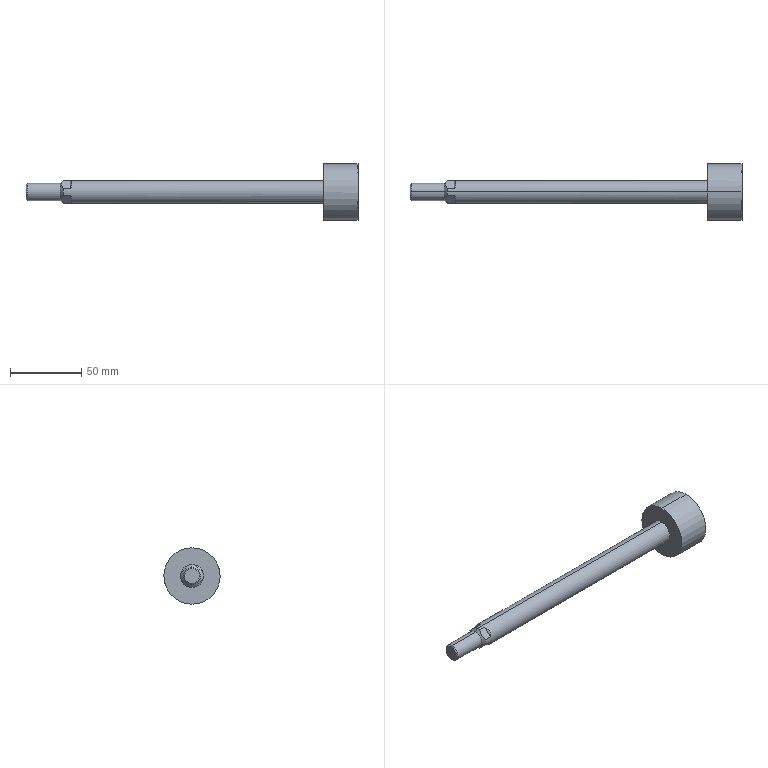Part | SolidWorks | features BaseBody 1 | 1 solid | 21 faces | box 232.5 x 39.5 x 39.5 mm | volume 68995 mm3 | plane 11 | cylinder 6 | cone 4 | commonest cylinder face diameters 12 x2 16 x2 39.5 x2
STEP:
#1=CARTESIAN_POINT('',(159.5,0.,-19.75));
#2=VERTEX_POINT('',#1);
#3=CARTESIAN_POINT('',(159.5,0.,19.75));
#4=VERTEX_POINT('',#3);
#5=CARTESIAN_POINT('',(159.5,0.,-19.75));
#6=CARTESIAN_POINT('',(159.5,1.293,-19.75));
#7=CARTESIAN_POINT('',(159.5,2.585,-19.623));
#8=CARTESIAN_POINT('',(159.5,5.121,-19.118));
#9=CARTESIAN_POINT('',(159.5,6.364,-18.741));
#10=CARTESIAN_POINT('',(159.5,8.752,-17.752));
#11=CARTESIAN_POINT('',(159.5,9.898,-17.14));
#12=CARTESIAN_POINT('',(159.5,12.047,-15.703));
#13=CARTESIAN_POINT('',(159.5,13.051,-14.879));
#14=CARTESIAN_POINT('',(159.5,14.879,-13.051));
#15=CARTESIAN_POINT('',(159.5,15.703,-12.047));
#16=CARTESIAN_POINT('',(159.5,17.14,-9.898));
#17=CARTESIAN_POINT('',(159.5,17.752,-8.752));
#18=CARTESIAN_POINT('',(159.5,18.741,-6.364));
#19=CARTESIAN_POINT('',(159.5,19.118,-5.121));
#20=CARTESIAN_POINT('',(159.5,19.623,-2.585));
#21=CARTESIAN_POINT('',(159.5,19.75,-1.293));
#22=CARTESIAN_POINT('',(159.5,19.75,1.293));
#23=CARTESIAN_POINT('',(159.5,19.623,2.585));
#24=CARTESIAN_POINT('',(159.5,19.118,5.121));
#25=CARTESIAN_POINT('',(159.5,18.741,6.364));
#26=CARTESIAN_POINT('',(159.5,17.752,8.752));
#27=CARTESIAN_POINT('',(159.5,17.14,9.898));
#28=CARTESIAN_POINT('',(159.5,15.703,12.047));
#29=CARTESIAN_POINT('',(159.5,14.879,13.051));
#30=CARTESIAN_POINT('',(159.5,13.051,14.879));
#31=CARTESIAN_POINT('',(159.5,12.047,15.703));
#32=CARTESIAN_POINT('',(159.5,9.898,17.14));
#33=CARTESIAN_POINT('',(159.5,8.752,17.752));
#34=CARTESIAN_POINT('',(159.5,6.364,18.741));
#35=CARTESIAN_POINT('',(159.5,5.121,19.118));
#36=CARTESIAN_POINT('',(159.5,2.585,19.623));
#37=CARTESIAN_POINT('',(159.5,1.293,19.75));
#38=CARTESIAN_POINT('',(159.5,0.,19.75));
#39=B_SPLINE_CURVE_WITH_KNOTS('',3,(#5,#6,#7,#8,#9,#10,#11,#12,#13,#14,#15,#16,#17,#18,#19,#20,#21,#22,#23,#24,#25,#26,#27,#28,#29,#30,#31,#32,#33,#34,#35,#36,#37,#38),.UNSPECIFIED.,.F.,.F.,(4,2,2,2,2,2,2,2,2,2,2,2,2,2,2,2,4),(0.,0.1963,0.3927,0.589,0.7854,0.9817,1.178,1.374,1.571,1.767,1.963,2.16,2.356,2.553,2.749,2.945,3.142),.UNSPECIFIED.);
#40=EDGE_CURVE('',#2,#4,#39,.T.);
#41=ORIENTED_EDGE('',*,*,#40,.T.);
#42=CARTESIAN_POINT('',(183.5,0.,19.75));
#43=VERTEX_POINT('',#42);
#44=CARTESIAN_POINT('',(183.5,0.,19.75));
#45=DIRECTION('',(1.,0.,0.));
#46=VECTOR('',#45,1000.);
#47=LINE('',#44,#46);
#48=EDGE_CURVE('',#4,#43,#47,.T.);
#49=ORIENTED_EDGE('',*,*,#48,.T.);
#50=CARTESIAN_POINT('',(183.5,0.,-19.75));
#51=VERTEX_POINT('',#50);
#52=CARTESIAN_POINT('',(183.5,0.,-19.75));
#53=CARTESIAN_POINT('',(183.5,1.297,-19.75));
#54=CARTESIAN_POINT('',(183.5,2.581,-19.624));
#55=CARTESIAN_POINT('',(183.5,5.125,-19.118));
#56=CARTESIAN_POINT('',(183.5,6.36,-18.743));
#57=CARTESIAN_POINT('',(183.5,8.756,-17.75));
#58=CARTESIAN_POINT('',(183.5,9.894,-17.142));
#59=CARTESIAN_POINT('',(183.5,12.051,-15.701));
#60=CARTESIAN_POINT('',(183.5,13.048,-14.882));
#61=CARTESIAN_POINT('',(183.5,14.882,-13.048));
#62=CARTESIAN_POINT('',(183.5,15.701,-12.051));
#63=CARTESIAN_POINT('',(183.5,17.142,-9.894));
#64=CARTESIAN_POINT('',(183.5,17.75,-8.756));
#65=CARTESIAN_POINT('',(183.5,18.743,-6.36));
#66=CARTESIAN_POINT('',(183.5,19.118,-5.125));
#67=CARTESIAN_POINT('',(183.5,19.624,-2.581));
#68=CARTESIAN_POINT('',(183.5,19.75,-1.297));
#69=CARTESIAN_POINT('',(183.5,19.75,1.297));
#70=CARTESIAN_POINT('',(183.5,19.624,2.581));
#71=CARTESIAN_POINT('',(183.5,19.118,5.125));
#72=CARTESIAN_POINT('',(183.5,18.743,6.36));
#73=CARTESIAN_POINT('',(183.5,17.75,8.756));
#74=CARTESIAN_POINT('',(183.5,17.142,9.894));
#75=CARTESIAN_POINT('',(183.5,15.701,12.051));
#76=CARTESIAN_POINT('',(183.5,14.882,13.048));
#77=CARTESIAN_POINT('',(183.5,13.048,14.882));
#78=CARTESIAN_POINT('',(183.5,12.051,15.701));
#79=CARTESIAN_POINT('',(183.5,9.894,17.142));
#80=CARTESIAN_POINT('',(183.5,8.756,17.75));
#81=CARTESIAN_POINT('',(183.5,6.36,18.743));
#82=CARTESIAN_POINT('',(183.5,5.125,19.118));
#83=CARTESIAN_POINT('',(183.5,2.581,19.624));
#84=CARTESIAN_POINT('',(183.5,1.297,19.75));
#85=CARTESIAN_POINT('',(183.5,0.,19.75));
#86=B_SPLINE_CURVE_WITH_KNOTS('',3,(#52,#53,#54,#55,#56,#57,#58,#59,#60,#61,#62,#63,#64,#65,#66,#67,#68,#69,#70,#71,#72,#73,#74,#75,#76,#77,#78,#79,#80,#81,#82,#83,#84,#85),.UNSPECIFIED.,.F.,.F.,(4,2,2,2,2,2,2,2,2,2,2,2,2,2,2,2,4),(0.,0.1963,0.3927,0.589,0.7854,0.9817,1.178,1.374,1.571,1.767,1.963,2.16,2.356,2.553,2.749,2.945,3.142),.UNSPECIFIED.);
#87=EDGE_CURVE('',#51,#43,#86,.T.);
#88=ORIENTED_EDGE('',*,*,#87,.F.);
#89=CARTESIAN_POINT('',(183.5,0.,-19.75));
#90=DIRECTION('',(1.,0.,0.));
#91=VECTOR('',#90,1000.);
#92=LINE('',#89,#91);
#93=EDGE_CURVE('',#2,#51,#92,.T.);
#94=ORIENTED_EDGE('',*,*,#93,.F.);
#95=EDGE_LOOP('',(#41,#49,#88,#94));
#96=FACE_OUTER_BOUND('',#95,.T.);
#97=CARTESIAN_POINT('',(183.5,0.,0.));
#98=DIRECTION('',(1.,0.,0.));
#99=DIRECTION('',(0.,0.,-1.));
#100=AXIS2_PLACEMENT_3D('',#97,#98,#99);
#101=CYLINDRICAL_SURFACE('',#100,19.75);
#102=ADVANCED_FACE('',(#96),#101,.T.);
#103=CARTESIAN_POINT('',(-48.233,0.,-6.));
#104=VERTEX_POINT('',#103);
#105=CARTESIAN_POINT('',(-48.233,0.,6.));
#106=VERTEX_POINT('',#105);
#107=CARTESIAN_POINT('',(-48.233,0.,-6.));
#108=CARTESIAN_POINT('',(-48.233,0.7854,-6.));
#109=CARTESIAN_POINT('',(-48.233,1.57,-5.844));
#110=CARTESIAN_POINT('',(-48.233,3.022,-5.243));
#111=CARTESIAN_POINT('',(-48.233,3.687,-4.798));
#112=CARTESIAN_POINT('',(-48.233,4.798,-3.687));
#113=CARTESIAN_POINT('',(-48.233,5.243,-3.022));
#114=CARTESIAN_POINT('',(-48.233,5.844,-1.57));
#115=CARTESIAN_POINT('',(-48.233,6.,-0.7854));
#116=CARTESIAN_POINT('',(-48.233,6.,0.7854));
#117=CARTESIAN_POINT('',(-48.233,5.844,1.57));
#118=CARTESIAN_POINT('',(-48.233,5.243,3.022));
#119=CARTESIAN_POINT('',(-48.233,4.798,3.687));
#120=CARTESIAN_POINT('',(-48.233,3.687,4.798));
#121=CARTESIAN_POINT('',(-48.233,3.022,5.243));
#122=CARTESIAN_POINT('',(-48.233,1.57,5.844));
#123=CARTESIAN_POINT('',(-48.233,0.7854,6.));
#124=CARTESIAN_POINT('',(-48.233,0.,6.));
#125=B_SPLINE_CURVE_WITH_KNOTS('',3,(#107,#108,#109,#110,#111,#112,#113,#114,#115,#116,#117,#118,#119,#120,#121,#122,#123,#124),.UNSPECIFIED.,.F.,.F.,(4,2,2,2,2,2,2,2,4),(0.,0.3927,0.7854,1.178,1.571,1.963,2.356,2.749,3.142),.UNSPECIFIED.);
#126=EDGE_CURVE('',#104,#106,#125,.T.);
#127=ORIENTED_EDGE('',*,*,#126,.T.);
#128=CARTESIAN_POINT('',(-25.,0.,6.));
#129=VERTEX_POINT('',#128);
#130=CARTESIAN_POINT('',(183.5,0.,6.));
#131=DIRECTION('',(1.,0.,0.));
#132=VECTOR('',#131,1000.);
#133=LINE('',#130,#132);
#134=EDGE_CURVE('',#106,#129,#133,.T.);
#135=ORIENTED_EDGE('',*,*,#134,.T.);
#136=CARTESIAN_POINT('',(-25.,0.,-6.));
#137=VERTEX_POINT('',#136);
#138=CARTESIAN_POINT('',(-25.,0.,-6.));
#139=CARTESIAN_POINT('',(-25.,0.7854,-6.));
#140=CARTESIAN_POINT('',(-25.,1.57,-5.844));
#141=CARTESIAN_POINT('',(-25.,3.022,-5.243));
#142=CARTESIAN_POINT('',(-25.,3.687,-4.798));
#143=CARTESIAN_POINT('',(-25.,4.798,-3.687));
#144=CARTESIAN_POINT('',(-25.,5.243,-3.022));
#145=CARTESIAN_POINT('',(-25.,5.844,-1.57));
#146=CARTESIAN_POINT('',(-25.,6.,-0.7854));
#147=CARTESIAN_POINT('',(-25.,6.,0.7854));
#148=CARTESIAN_POINT('',(-25.,5.844,1.57));
#149=CARTESIAN_POINT('',(-25.,5.243,3.022));
#150=CARTESIAN_POINT('',(-25.,4.798,3.687));
#151=CARTESIAN_POINT('',(-25.,3.687,4.798));
#152=CARTESIAN_POINT('',(-25.,3.022,5.243));
#153=CARTESIAN_POINT('',(-25.,1.57,5.844));
#154=CARTESIAN_POINT('',(-25.,0.7854,6.));
#155=CARTESIAN_POINT('',(-25.,0.,6.));
#156=B_SPLINE_CURVE_WITH_KNOTS('',3,(#138,#139,#140,#141,#142,#143,#144,#145,#146,#147,#148,#149,#150,#151,#152,#153,#154,#155),.UNSPECIFIED.,.F.,.F.,(4,2,2,2,2,2,2,2,4),(0.,0.3927,0.7854,1.178,1.571,1.963,2.356,2.749,3.142),.UNSPECIFIED.);
#157=EDGE_CURVE('',#137,#129,#156,.T.);
#158=ORIENTED_EDGE('',*,*,#157,.F.);
#159=CARTESIAN_POINT('',(183.5,0.,-6.));
#160=DIRECTION('',(1.,0.,0.));
#161=VECTOR('',#160,1000.);
#162=LINE('',#159,#161);
#163=EDGE_CURVE('',#104,#137,#162,.T.);
#164=ORIENTED_EDGE('',*,*,#163,.F.);
#165=EDGE_LOOP('',(#127,#135,#158,#164));
#166=FACE_OUTER_BOUND('',#165,.T.);
#167=CARTESIAN_POINT('',(183.5,0.,0.));
#168=DIRECTION('',(1.,0.,0.));
#169=DIRECTION('',(0.,0.,-1.));
#170=AXIS2_PLACEMENT_3D('',#167,#168,#169);
#171=CYLINDRICAL_SURFACE('',#170,6.);
#172=ADVANCED_FACE('',(#166),#171,.T.);
#173=CARTESIAN_POINT('',(-49.,0.,-5.233));
#174=VERTEX_POINT('',#173);
#175=CARTESIAN_POINT('',(-49.,0.,5.233));
#176=VERTEX_POINT('',#175);
#177=CARTESIAN_POINT('',(-49.,0.,-5.233));
#178=CARTESIAN_POINT('',(-49.,0.685,-5.233));
#179=CARTESIAN_POINT('',(-49.,1.37,-5.097));
#180=CARTESIAN_POINT('',(-49.,2.635,-4.573));
#181=CARTESIAN_POINT('',(-49.,3.216,-4.185));
#182=CARTESIAN_POINT('',(-49.,4.185,-3.216));
#183=CARTESIAN_POINT('',(-49.,4.573,-2.635));
#184=CARTESIAN_POINT('',(-49.,5.097,-1.37));
#185=CARTESIAN_POINT('',(-49.,5.233,-0.685));
#186=CARTESIAN_POINT('',(-49.,5.233,0.685));
#187=CARTESIAN_POINT('',(-49.,5.097,1.37));
#188=CARTESIAN_POINT('',(-49.,4.573,2.635));
#189=CARTESIAN_POINT('',(-49.,4.185,3.216));
#190=CARTESIAN_POINT('',(-49.,3.216,4.185));
#191=CARTESIAN_POINT('',(-49.,2.635,4.573));
#192=CARTESIAN_POINT('',(-49.,1.37,5.097));
#193=CARTESIAN_POINT('',(-49.,0.685,5.233));
#194=CARTESIAN_POINT('',(-49.,0.,5.233));
#195=B_SPLINE_CURVE_WITH_KNOTS('',3,(#177,#178,#179,#180,#181,#182,#183,#184,#185,#186,#187,#188,#189,#190,#191,#192,#193,#194),.UNSPECIFIED.,.F.,.F.,(4,2,2,2,2,2,2,2,4),(0.,0.3927,0.7854,1.178,1.571,1.963,2.356,2.749,3.142),.UNSPECIFIED.);
#196=EDGE_CURVE('',#174,#176,#195,.T.);
#197=ORIENTED_EDGE('',*,*,#196,.T.);
#198=CARTESIAN_POINT('',(-49.,0.,5.233));
#199=DIRECTION('',(0.7071,0.,0.7071));
#200=VECTOR('',#199,1000.);
#201=LINE('',#198,#200);
#202=EDGE_CURVE('',#176,#106,#201,.T.);
#203=ORIENTED_EDGE('',*,*,#202,.T.);
#204=ORIENTED_EDGE('',*,*,#126,.F.);
#205=CARTESIAN_POINT('',(-49.,0.,-5.233));
#206=DIRECTION('',(0.7071,0.,-0.7071));
#207=VECTOR('',#206,1000.);
#208=LINE('',#205,#207);
#209=EDGE_CURVE('',#174,#104,#208,.T.);
#210=ORIENTED_EDGE('',*,*,#209,.F.);
#211=EDGE_LOOP('',(#197,#203,#204,#210));
#212=FACE_OUTER_BOUND('',#211,.T.);
#213=CARTESIAN_POINT('',(-49.,0.,0.));
#214=DIRECTION('',(1.,0.,0.));
#215=DIRECTION('',(0.,0.,-1.));
#216=AXIS2_PLACEMENT_3D('',#213,#214,#215);
#217=CONICAL_SURFACE('',#216,5.233,0.7854);
#218=ADVANCED_FACE('',(#212),#217,.T.);
#219=CARTESIAN_POINT('',(-23.,2.211,7.688));
#220=VERTEX_POINT('',#219);
#221=CARTESIAN_POINT('',(-23.,0.,8.));
#222=VERTEX_POINT('',#221);
#223=CARTESIAN_POINT('',(-23.,0.,0.));
#224=DIRECTION('',(1.,0.,0.));
#225=DIRECTION('',(0.,0.2764,0.961));
#226=AXIS2_PLACEMENT_3D('',#223,#224,#225);
#227=CIRCLE('',#226,8.);
#228=EDGE_CURVE('',#220,#222,#227,.T.);
#229=ORIENTED_EDGE('',*,*,#228,.T.);
#230=CARTESIAN_POINT('',(159.5,0.,8.));
#231=VERTEX_POINT('',#230);
#232=CARTESIAN_POINT('',(183.5,0.,8.));
#233=DIRECTION('',(1.,0.,0.));
#234=VECTOR('',#233,1000.);
#235=LINE('',#232,#234);
#236=EDGE_CURVE('',#222,#231,#235,.T.);
#237=ORIENTED_EDGE('',*,*,#236,.T.);
#238=CARTESIAN_POINT('',(159.5,0.,-8.));
#239=VERTEX_POINT('',#238);
#240=CARTESIAN_POINT('',(159.5,0.,-8.));
#241=CARTESIAN_POINT('',(159.5,0.5253,-8.));
#242=CARTESIAN_POINT('',(159.5,1.046,-7.949));
#243=CARTESIAN_POINT('',(159.5,2.076,-7.744));
#244=CARTESIAN_POINT('',(159.5,2.576,-7.592));
#245=CARTESIAN_POINT('',(159.5,3.547,-7.19));
#246=CARTESIAN_POINT('',(159.5,4.008,-6.944));
#247=CARTESIAN_POINT('',(159.5,4.881,-6.36));
#248=CARTESIAN_POINT('',(159.5,5.285,-6.028));
#249=CARTESIAN_POINT('',(159.5,6.028,-5.285));
#250=CARTESIAN_POINT('',(159.5,6.36,-4.881));
#251=CARTESIAN_POINT('',(159.5,6.944,-4.008));
#252=CARTESIAN_POINT('',(159.5,7.19,-3.547));
#253=CARTESIAN_POINT('',(159.5,7.592,-2.576));
#254=CARTESIAN_POINT('',(159.5,7.744,-2.076));
#255=CARTESIAN_POINT('',(159.5,7.949,-1.046));
#256=CARTESIAN_POINT('',(159.5,8.,-0.5253));
#257=CARTESIAN_POINT('',(159.5,8.,0.5253));
#258=CARTESIAN_POINT('',(159.5,7.949,1.046));
#259=CARTESIAN_POINT('',(159.5,7.744,2.076));
#260=CARTESIAN_POINT('',(159.5,7.592,2.576));
#261=CARTESIAN_POINT('',(159.5,7.19,3.547));
#262=CARTESIAN_POINT('',(159.5,6.944,4.008));
#263=CARTESIAN_POINT('',(159.5,6.36,4.881));
#264=CARTESIAN_POINT('',(159.5,6.028,5.285));
#265=CARTESIAN_POINT('',(159.5,5.285,6.028));
#266=CARTESIAN_POINT('',(159.5,4.881,6.36));
#267=CARTESIAN_POINT('',(159.5,4.008,6.944));
#268=CARTESIAN_POINT('',(159.5,3.547,7.19));
#269=CARTESIAN_POINT('',(159.5,2.576,7.592));
#270=CARTESIAN_POINT('',(159.5,2.076,7.744));
#271=CARTESIAN_POINT('',(159.5,1.046,7.949));
#272=CARTESIAN_POINT('',(159.5,0.5253,8.));
#273=CARTESIAN_POINT('',(159.5,0.,8.));
#274=B_SPLINE_CURVE_WITH_KNOTS('',3,(#240,#241,#242,#243,#244,#245,#246,#247,#248,#249,#250,#251,#252,#253,#254,#255,#256,#257,#258,#259,#260,#261,#262,#263,#264,#265,#266,#267,#268,#269,#270,#271,#272,#273),.UNSPECIFIED.,.F.,.F.,(4,2,2,2,2,2,2,2,2,2,2,2,2,2,2,2,4),(0.,0.1963,0.3927,0.589,0.7854,0.9817,1.178,1.374,1.571,1.767,1.963,2.16,2.356,2.553,2.749,2.945,3.142),.UNSPECIFIED.);
#275=EDGE_CURVE('',#239,#231,#274,.T.);
#276=ORIENTED_EDGE('',*,*,#275,.F.);
#277=CARTESIAN_POINT('',(-23.,0.,-8.));
#278=VERTEX_POINT('',#277);
#279=CARTESIAN_POINT('',(183.5,0.,-8.));
#280=DIRECTION('',(1.,0.,0.));
#281=VECTOR('',#280,1000.);
#282=LINE('',#279,#281);
#283=EDGE_CURVE('',#278,#239,#282,.T.);
#284=ORIENTED_EDGE('',*,*,#283,.F.);
#285=CARTESIAN_POINT('',(-23.,2.211,-7.688));
#286=VERTEX_POINT('',#285);
#287=CARTESIAN_POINT('',(-23.,0.,0.));
#288=DIRECTION('',(1.,0.,0.));
#289=DIRECTION('',(0.,-0.2764,-0.961));
#290=AXIS2_PLACEMENT_3D('',#287,#288,#289);
#291=CIRCLE('',#290,8.);
#292=EDGE_CURVE('',#278,#286,#291,.T.);
#293=ORIENTED_EDGE('',*,*,#292,.T.);
#294=CARTESIAN_POINT('',(-18.,2.211,-7.688));
#295=VERTEX_POINT('',#294);
#296=CARTESIAN_POINT('',(-18.,2.211,-7.688));
#297=DIRECTION('',(-1.,0.,0.));
#298=VECTOR('',#297,1000.);
#299=LINE('',#296,#298);
#300=EDGE_CURVE('',#295,#286,#299,.T.);
#301=ORIENTED_EDGE('',*,*,#300,.F.);
#302=CARTESIAN_POINT('',(-18.,7.688,-2.211));
#303=VERTEX_POINT('',#302);
#304=CARTESIAN_POINT('',(-18.,7.688,-2.211));
#305=CARTESIAN_POINT('',(-17.842,7.598,-2.525));
#306=CARTESIAN_POINT('',(-17.628,7.434,-2.991));
#307=CARTESIAN_POINT('',(-17.425,7.183,-3.53));
#308=CARTESIAN_POINT('',(-17.335,7.043,-3.797));
#309=CARTESIAN_POINT('',(-17.294,6.968,-3.93));
#310=CARTESIAN_POINT('',(-17.276,6.936,-3.987));
#311=CARTESIAN_POINT('',(-17.265,6.914,-4.025));
#312=CARTESIAN_POINT('',(-17.259,6.902,-4.045));
#313=CARTESIAN_POINT('',(-17.087,6.553,-4.638));
#314=CARTESIAN_POINT('',(-17.,6.143,-5.17));
#315=CARTESIAN_POINT('',(-17.,5.414,-5.9));
#316=CARTESIAN_POINT('',(-17.033,5.031,-6.236));
#317=CARTESIAN_POINT('',(-17.126,4.557,-6.58));
#318=CARTESIAN_POINT('',(-17.185,4.312,-6.739));
#319=CARTESIAN_POINT('',(-17.219,4.188,-6.816));
#320=CARTESIAN_POINT('',(-17.234,4.135,-6.849));
#321=CARTESIAN_POINT('',(-17.244,4.099,-6.87));
#322=CARTESIAN_POINT('',(-17.249,4.082,-6.88));
#323=CARTESIAN_POINT('',(-17.43,3.456,-7.249));
#324=CARTESIAN_POINT('',(-17.684,2.838,-7.508));
#325=CARTESIAN_POINT('',(-18.,2.211,-7.688));
#326=B_SPLINE_CURVE_WITH_KNOTS('',3,(#304,#305,#306,#307,#308,#309,#310,#311,#312,#313,#314,#315,#316,#317,#318,#319,#320,#321,#322,#323,#324,#325),.UNSPECIFIED.,.F.,.F.,(4,1,1,1,1,2,2,2,1,1,1,1,2,2,4),(5.778,5.904,5.967,5.999,6.015,6.023,6.031,6.283,6.41,6.473,6.504,6.52,6.528,6.536,6.789),.UNSPECIFIED.);
#327=EDGE_CURVE('',#303,#295,#326,.T.);
#328=ORIENTED_EDGE('',*,*,#327,.F.);
#329=CARTESIAN_POINT('',(-23.,7.688,-2.211));
#330=VERTEX_POINT('',#329);
#331=CARTESIAN_POINT('',(-23.,7.688,-2.211));
#332=DIRECTION('',(1.,0.,0.));
#333=VECTOR('',#332,1000.);
#334=LINE('',#331,#333);
#335=EDGE_CURVE('',#330,#303,#334,.T.);
#336=ORIENTED_EDGE('',*,*,#335,.F.);
#337=CARTESIAN_POINT('',(-23.,7.688,2.211));
#338=VERTEX_POINT('',#337);
#339=CARTESIAN_POINT('',(-23.,0.,0.));
#340=DIRECTION('',(1.,0.,0.));
#341=DIRECTION('',(0.,0.961,-0.2764));
#342=AXIS2_PLACEMENT_3D('',#339,#340,#341);
#343=CIRCLE('',#342,8.);
#344=EDGE_CURVE('',#330,#338,#343,.T.);
#345=ORIENTED_EDGE('',*,*,#344,.T.);
#346=CARTESIAN_POINT('',(-18.,7.688,2.211));
#347=VERTEX_POINT('',#346);
#348=CARTESIAN_POINT('',(-18.,7.688,2.211));
#349=DIRECTION('',(-1.,0.,0.));
#350=VECTOR('',#349,1000.);
#351=LINE('',#348,#350);
#352=EDGE_CURVE('',#347,#338,#351,.T.);
#353=ORIENTED_EDGE('',*,*,#352,.F.);
#354=CARTESIAN_POINT('',(-18.,2.211,7.688));
#355=VERTEX_POINT('',#354);
#356=CARTESIAN_POINT('',(-18.,2.211,7.688));
#357=CARTESIAN_POINT('',(-17.842,2.525,7.598));
#358=CARTESIAN_POINT('',(-17.628,2.991,7.434));
#359=CARTESIAN_POINT('',(-17.425,3.53,7.183));
#360=CARTESIAN_POINT('',(-17.335,3.797,7.043));
#361=CARTESIAN_POINT('',(-17.294,3.93,6.968));
#362=CARTESIAN_POINT('',(-17.276,3.987,6.936));
#363=CARTESIAN_POINT('',(-17.265,4.025,6.914));
#364=CARTESIAN_POINT('',(-17.259,4.045,6.902));
#365=CARTESIAN_POINT('',(-17.087,4.638,6.553));
#366=CARTESIAN_POINT('',(-17.,5.17,6.143));
#367=CARTESIAN_POINT('',(-17.,5.9,5.414));
#368=CARTESIAN_POINT('',(-17.033,6.236,5.031));
#369=CARTESIAN_POINT('',(-17.126,6.58,4.557));
#370=CARTESIAN_POINT('',(-17.185,6.739,4.312));
#371=CARTESIAN_POINT('',(-17.219,6.816,4.188));
#372=CARTESIAN_POINT('',(-17.234,6.849,4.135));
#373=CARTESIAN_POINT('',(-17.244,6.87,4.099));
#374=CARTESIAN_POINT('',(-17.249,6.88,4.082));
#375=CARTESIAN_POINT('',(-17.43,7.249,3.456));
#376=CARTESIAN_POINT('',(-17.684,7.508,2.838));
#377=CARTESIAN_POINT('',(-18.,7.688,2.211));
#378=B_SPLINE_CURVE_WITH_KNOTS('',3,(#356,#357,#358,#359,#360,#361,#362,#363,#364,#365,#366,#367,#368,#369,#370,#371,#372,#373,#374,#375,#376,#377),.UNSPECIFIED.,.F.,.F.,(4,1,1,1,1,2,2,2,1,1,1,1,2,2,4),(5.778,5.904,5.967,5.999,6.015,6.023,6.031,6.283,6.41,6.473,6.504,6.52,6.528,6.536,6.789),.UNSPECIFIED.);
#379=EDGE_CURVE('',#355,#347,#378,.T.);
#380=ORIENTED_EDGE('',*,*,#379,.F.);
#381=CARTESIAN_POINT('',(-23.,2.211,7.688));
#382=DIRECTION('',(1.,0.,0.));
#383=VECTOR('',#382,1000.);
#384=LINE('',#381,#383);
#385=EDGE_CURVE('',#220,#355,#384,.T.);
#386=ORIENTED_EDGE('',*,*,#385,.F.);
#387=EDGE_LOOP('',(#229,#237,#276,#284,#293,#301,#328,#336,#345,#353,#380,#386));
#388=FACE_OUTER_BOUND('',#387,.T.);
#389=CARTESIAN_POINT('',(183.5,0.,0.));
#390=DIRECTION('',(1.,0.,0.));
#391=DIRECTION('',(0.,0.,-1.));
#392=AXIS2_PLACEMENT_3D('',#389,#390,#391);
#393=CYLINDRICAL_SURFACE('',#392,8.);
#394=ADVANCED_FACE('',(#388),#393,.T.);
#395=ORIENTED_EDGE('',*,*,#157,.T.);
#396=CARTESIAN_POINT('',(-25.,0.,6.));
#397=DIRECTION('',(0.7071,0.,0.7071));
#398=VECTOR('',#397,1000.);
#399=LINE('',#396,#398);
#400=EDGE_CURVE('',#129,#222,#399,.T.);
#401=ORIENTED_EDGE('',*,*,#400,.T.);
#402=ORIENTED_EDGE('',*,*,#228,.F.);
#403=CARTESIAN_POINT('',(-23.,7.688,2.211));
#404=CARTESIAN_POINT('',(-23.292,7.262,2.638));
#405=CARTESIAN_POINT('',(-23.542,6.822,3.077));
#406=CARTESIAN_POINT('',(-23.808,6.136,3.763));
#407=CARTESIAN_POINT('',(-23.878,5.905,3.995));
#408=CARTESIAN_POINT('',(-23.974,5.437,4.463));
#409=CARTESIAN_POINT('',(-23.999,5.198,4.701));
#410=CARTESIAN_POINT('',(-24.001,4.723,5.177));
#411=CARTESIAN_POINT('',(-23.977,4.485,5.415));
#412=CARTESIAN_POINT('',(-23.883,4.013,5.887));
#413=CARTESIAN_POINT('',(-23.814,3.78,6.119));
#414=CARTESIAN_POINT('',(-23.637,3.321,6.579));
#415=CARTESIAN_POINT('',(-23.529,3.092,6.807));
#416=CARTESIAN_POINT('',(-23.285,2.646,7.253));
#417=CARTESIAN_POINT('',(-23.148,2.427,7.472));
#418=CARTESIAN_POINT('',(-23.,2.211,7.688));
#419=B_SPLINE_CURVE_WITH_KNOTS('',3,(#403,#404,#405,#406,#407,#408,#409,#410,#411,#412,#413,#414,#415,#416,#417,#418),.UNSPECIFIED.,.F.,.F.,(4,2,2,2,2,2,2,4),(0.0004524,1.997,2.995,3.993,4.991,5.989,6.987,7.985),.UNSPECIFIED.);
#420=EDGE_CURVE('',#338,#220,#419,.T.);
#421=ORIENTED_EDGE('',*,*,#420,.F.);
#422=ORIENTED_EDGE('',*,*,#344,.F.);
#423=CARTESIAN_POINT('',(-23.,2.211,-7.688));
#424=CARTESIAN_POINT('',(-23.292,2.638,-7.262));
#425=CARTESIAN_POINT('',(-23.542,3.077,-6.822));
#426=CARTESIAN_POINT('',(-23.808,3.763,-6.136));
#427=CARTESIAN_POINT('',(-23.878,3.995,-5.905));
#428=CARTESIAN_POINT('',(-23.974,4.463,-5.437));
#429=CARTESIAN_POINT('',(-23.999,4.701,-5.198));
#430=CARTESIAN_POINT('',(-24.001,5.177,-4.723));
#431=CARTESIAN_POINT('',(-23.977,5.415,-4.485));
#432=CARTESIAN_POINT('',(-23.883,5.887,-4.013));
#433=CARTESIAN_POINT('',(-23.814,6.119,-3.78));
#434=CARTESIAN_POINT('',(-23.637,6.579,-3.321));
#435=CARTESIAN_POINT('',(-23.529,6.807,-3.092));
#436=CARTESIAN_POINT('',(-23.285,7.253,-2.646));
#437=CARTESIAN_POINT('',(-23.148,7.472,-2.427));
#438=CARTESIAN_POINT('',(-23.,7.688,-2.211));
#439=B_SPLINE_CURVE_WITH_KNOTS('',3,(#423,#424,#425,#426,#427,#428,#429,#430,#431,#432,#433,#434,#435,#436,#437,#438),.UNSPECIFIED.,.F.,.F.,(4,2,2,2,2,2,2,4),(0.0004524,1.997,2.995,3.993,4.991,5.989,6.987,7.985),.UNSPECIFIED.);
#440=EDGE_CURVE('',#286,#330,#439,.T.);
#441=ORIENTED_EDGE('',*,*,#440,.F.);
#442=ORIENTED_EDGE('',*,*,#292,.F.);
#443=CARTESIAN_POINT('',(-25.,0.,-6.));
#444=DIRECTION('',(0.7071,0.,-0.7071));
#445=VECTOR('',#444,1000.);
#446=LINE('',#443,#445);
#447=EDGE_CURVE('',#137,#278,#446,.T.);
#448=ORIENTED_EDGE('',*,*,#447,.F.);
#449=EDGE_LOOP('',(#395,#401,#402,#421,#422,#441,#442,#448));
#450=FACE_OUTER_BOUND('',#449,.T.);
#451=CARTESIAN_POINT('',(-25.,0.,0.));
#452=DIRECTION('',(1.,0.,0.));
#453=DIRECTION('',(0.,0.,-1.));
#454=AXIS2_PLACEMENT_3D('',#451,#452,#453);
#455=CONICAL_SURFACE('',#454,6.,0.7854);
#456=ADVANCED_FACE('',(#450),#455,.T.);
#457=ORIENTED_EDGE('',*,*,#400,.F.);
#458=CARTESIAN_POINT('',(-25.,0.,6.));
#459=CARTESIAN_POINT('',(-25.,-0.7854,6.));
#460=CARTESIAN_POINT('',(-25.,-1.57,5.844));
#461=CARTESIAN_POINT('',(-25.,-3.022,5.243));
#462=CARTESIAN_POINT('',(-25.,-3.687,4.798));
#463=CARTESIAN_POINT('',(-25.,-4.798,3.687));
#464=CARTESIAN_POINT('',(-25.,-5.243,3.022));
#465=CARTESIAN_POINT('',(-25.,-5.844,1.57));
#466=CARTESIAN_POINT('',(-25.,-6.,0.7854));
#467=CARTESIAN_POINT('',(-25.,-6.,-0.7854));
#468=CARTESIAN_POINT('',(-25.,-5.844,-1.57));
#469=CARTESIAN_POINT('',(-25.,-5.243,-3.022));
#470=CARTESIAN_POINT('',(-25.,-4.798,-3.687));
#471=CARTESIAN_POINT('',(-25.,-3.687,-4.798));
#472=CARTESIAN_POINT('',(-25.,-3.022,-5.243));
#473=CARTESIAN_POINT('',(-25.,-1.57,-5.844));
#474=CARTESIAN_POINT('',(-25.,-0.7854,-6.));
#475=CARTESIAN_POINT('',(-25.,0.,-6.));
#476=B_SPLINE_CURVE_WITH_KNOTS('',3,(#458,#459,#460,#461,#462,#463,#464,#465,#466,#467,#468,#469,#470,#471,#472,#473,#474,#475),.UNSPECIFIED.,.F.,.F.,(4,2,2,2,2,2,2,2,4),(3.142,3.534,3.927,4.32,4.712,5.105,5.498,5.89,6.283),.UNSPECIFIED.);
#477=EDGE_CURVE('',#129,#137,#476,.T.);
#478=ORIENTED_EDGE('',*,*,#477,.T.);
#479=ORIENTED_EDGE('',*,*,#447,.T.);
#480=CARTESIAN_POINT('',(-23.,-2.211,-7.688));
#481=VERTEX_POINT('',#480);
#482=CARTESIAN_POINT('',(-23.,0.,0.));
#483=DIRECTION('',(1.,0.,0.));
#484=DIRECTION('',(0.,-0.2764,-0.961));
#485=AXIS2_PLACEMENT_3D('',#482,#483,#484);
#486=CIRCLE('',#485,8.);
#487=EDGE_CURVE('',#481,#278,#486,.T.);
#488=ORIENTED_EDGE('',*,*,#487,.F.);
#489=CARTESIAN_POINT('',(-23.,-7.688,-2.211));
#490=VERTEX_POINT('',#489);
#491=CARTESIAN_POINT('',(-23.,-7.688,-2.211));
#492=CARTESIAN_POINT('',(-23.292,-7.262,-2.638));
#493=CARTESIAN_POINT('',(-23.542,-6.822,-3.077));
#494=CARTESIAN_POINT('',(-23.808,-6.136,-3.763));
#495=CARTESIAN_POINT('',(-23.878,-5.905,-3.995));
#496=CARTESIAN_POINT('',(-23.974,-5.437,-4.463));
#497=CARTESIAN_POINT('',(-23.999,-5.198,-4.701));
#498=CARTESIAN_POINT('',(-24.001,-4.723,-5.177));
#499=CARTESIAN_POINT('',(-23.977,-4.485,-5.415));
#500=CARTESIAN_POINT('',(-23.883,-4.013,-5.887));
#501=CARTESIAN_POINT('',(-23.814,-3.78,-6.119));
#502=CARTESIAN_POINT('',(-23.637,-3.321,-6.579));
#503=CARTESIAN_POINT('',(-23.529,-3.092,-6.807));
#504=CARTESIAN_POINT('',(-23.285,-2.646,-7.253));
#505=CARTESIAN_POINT('',(-23.148,-2.427,-7.472));
#506=CARTESIAN_POINT('',(-23.,-2.211,-7.688));
#507=B_SPLINE_CURVE_WITH_KNOTS('',3,(#491,#492,#493,#494,#495,#496,#497,#498,#499,#500,#501,#502,#503,#504,#505,#506),.UNSPECIFIED.,.F.,.F.,(4,2,2,2,2,2,2,4),(0.0004524,1.997,2.995,3.993,4.991,5.989,6.987,7.985),.UNSPECIFIED.);
#508=EDGE_CURVE('',#490,#481,#507,.T.);
#509=ORIENTED_EDGE('',*,*,#508,.F.);
#510=CARTESIAN_POINT('',(-23.,-7.688,2.211));
#511=VERTEX_POINT('',#510);
#512=CARTESIAN_POINT('',(-23.,0.,0.));
#513=DIRECTION('',(1.,0.,0.));
#514=DIRECTION('',(0.,-0.961,0.2764));
#515=AXIS2_PLACEMENT_3D('',#512,#513,#514);
#516=CIRCLE('',#515,8.);
#517=EDGE_CURVE('',#511,#490,#516,.T.);
#518=ORIENTED_EDGE('',*,*,#517,.F.);
#519=CARTESIAN_POINT('',(-23.,-2.211,7.688));
#520=VERTEX_POINT('',#519);
#521=CARTESIAN_POINT('',(-23.,-2.211,7.688));
#522=CARTESIAN_POINT('',(-23.292,-2.638,7.262));
#523=CARTESIAN_POINT('',(-23.542,-3.077,6.822));
#524=CARTESIAN_POINT('',(-23.808,-3.763,6.136));
#525=CARTESIAN_POINT('',(-23.878,-3.995,5.905));
#526=CARTESIAN_POINT('',(-23.974,-4.463,5.437));
#527=CARTESIAN_POINT('',(-23.999,-4.701,5.198));
#528=CARTESIAN_POINT('',(-24.001,-5.177,4.723));
#529=CARTESIAN_POINT('',(-23.977,-5.415,4.485));
#530=CARTESIAN_POINT('',(-23.883,-5.887,4.013));
#531=CARTESIAN_POINT('',(-23.814,-6.119,3.78));
#532=CARTESIAN_POINT('',(-23.637,-6.579,3.321));
#533=CARTESIAN_POINT('',(-23.529,-6.807,3.092));
#534=CARTESIAN_POINT('',(-23.285,-7.253,2.646));
#535=CARTESIAN_POINT('',(-23.148,-7.472,2.427));
#536=CARTESIAN_POINT('',(-23.,-7.688,2.211));
#537=B_SPLINE_CURVE_WITH_KNOTS('',3,(#521,#522,#523,#524,#525,#526,#527,#528,#529,#530,#531,#532,#533,#534,#535,#536),.UNSPECIFIED.,.F.,.F.,(4,2,2,2,2,2,2,4),(0.0004524,1.997,2.995,3.993,4.991,5.989,6.987,7.985),.UNSPECIFIED.);
#538=EDGE_CURVE('',#520,#511,#537,.T.);
#539=ORIENTED_EDGE('',*,*,#538,.F.);
#540=CARTESIAN_POINT('',(-23.,0.,0.));
#541=DIRECTION('',(1.,0.,0.));
#542=DIRECTION('',(0.,0.2764,0.961));
#543=AXIS2_PLACEMENT_3D('',#540,#541,#542);
#544=CIRCLE('',#543,8.);
#545=EDGE_CURVE('',#222,#520,#544,.T.);
#546=ORIENTED_EDGE('',*,*,#545,.F.);
#547=EDGE_LOOP('',(#457,#478,#479,#488,#509,#518,#539,#546));
#548=FACE_OUTER_BOUND('',#547,.T.);
#549=CARTESIAN_POINT('',(-25.,0.,0.));
#550=DIRECTION('',(1.,0.,0.));
#551=DIRECTION('',(0.,0.,-1.));
#552=AXIS2_PLACEMENT_3D('',#549,#550,#551);
#553=CONICAL_SURFACE('',#552,6.,0.7854);
#554=ADVANCED_FACE('',(#548),#553,.T.);
#555=ORIENTED_EDGE('',*,*,#236,.F.);
#556=ORIENTED_EDGE('',*,*,#545,.T.);
#557=CARTESIAN_POINT('',(-18.,-2.211,7.688));
#558=VERTEX_POINT('',#557);
#559=CARTESIAN_POINT('',(-18.,-2.211,7.688));
#560=DIRECTION('',(-1.,0.,0.));
#561=VECTOR('',#560,1000.);
#562=LINE('',#559,#561);
#563=EDGE_CURVE('',#558,#520,#562,.T.);
#564=ORIENTED_EDGE('',*,*,#563,.F.);
#565=CARTESIAN_POINT('',(-18.,-7.688,2.211));
#566=VERTEX_POINT('',#565);
#567=CARTESIAN_POINT('',(-18.,-7.688,2.211));
#568=CARTESIAN_POINT('',(-17.842,-7.598,2.525));
#569=CARTESIAN_POINT('',(-17.628,-7.434,2.991));
#570=CARTESIAN_POINT('',(-17.425,-7.183,3.53));
#571=CARTESIAN_POINT('',(-17.335,-7.043,3.797));
#572=CARTESIAN_POINT('',(-17.294,-6.968,3.93));
#573=CARTESIAN_POINT('',(-17.276,-6.936,3.987));
#574=CARTESIAN_POINT('',(-17.265,-6.914,4.025));
#575=CARTESIAN_POINT('',(-17.259,-6.902,4.045));
#576=CARTESIAN_POINT('',(-17.087,-6.553,4.638));
#577=CARTESIAN_POINT('',(-17.,-6.143,5.17));
#578=CARTESIAN_POINT('',(-17.,-5.414,5.9));
#579=CARTESIAN_POINT('',(-17.033,-5.031,6.236));
#580=CARTESIAN_POINT('',(-17.126,-4.557,6.58));
#581=CARTESIAN_POINT('',(-17.185,-4.312,6.739));
#582=CARTESIAN_POINT('',(-17.219,-4.188,6.816));
#583=CARTESIAN_POINT('',(-17.234,-4.135,6.849));
#584=CARTESIAN_POINT('',(-17.244,-4.099,6.87));
#585=CARTESIAN_POINT('',(-17.249,-4.082,6.88));
#586=CARTESIAN_POINT('',(-17.43,-3.456,7.249));
#587=CARTESIAN_POINT('',(-17.684,-2.838,7.508));
#588=CARTESIAN_POINT('',(-18.,-2.211,7.688));
#589=B_SPLINE_CURVE_WITH_KNOTS('',3,(#567,#568,#569,#570,#571,#572,#573,#574,#575,#576,#577,#578,#579,#580,#581,#582,#583,#584,#585,#586,#587,#588),.UNSPECIFIED.,.F.,.F.,(4,1,1,1,1,2,2,2,1,1,1,1,2,2,4),(5.778,5.904,5.967,5.999,6.015,6.023,6.031,6.283,6.41,6.473,6.504,6.52,6.528,6.536,6.789),.UNSPECIFIED.);
#590=EDGE_CURVE('',#566,#558,#589,.T.);
#591=ORIENTED_EDGE('',*,*,#590,.F.);
#592=CARTESIAN_POINT('',(-23.,-7.688,2.211));
#593=DIRECTION('',(1.,0.,0.));
#594=VECTOR('',#593,1000.);
#595=LINE('',#592,#594);
#596=EDGE_CURVE('',#511,#566,#595,.T.);
#597=ORIENTED_EDGE('',*,*,#596,.F.);
#598=ORIENTED_EDGE('',*,*,#517,.T.);
#599=CARTESIAN_POINT('',(-18.,-7.688,-2.211));
#600=VERTEX_POINT('',#599);
#601=CARTESIAN_POINT('',(-18.,-7.688,-2.211));
#602=DIRECTION('',(-1.,0.,0.));
#603=VECTOR('',#602,1000.);
#604=LINE('',#601,#603);
#605=EDGE_CURVE('',#600,#490,#604,.T.);
#606=ORIENTED_EDGE('',*,*,#605,.F.);
#607=CARTESIAN_POINT('',(-18.,-2.211,-7.688));
#608=VERTEX_POINT('',#607);
#609=CARTESIAN_POINT('',(-18.,-2.211,-7.688));
#610=CARTESIAN_POINT('',(-17.842,-2.525,-7.598));
#611=CARTESIAN_POINT('',(-17.628,-2.991,-7.434));
#612=CARTESIAN_POINT('',(-17.425,-3.53,-7.183));
#613=CARTESIAN_POINT('',(-17.335,-3.797,-7.043));
#614=CARTESIAN_POINT('',(-17.294,-3.93,-6.968));
#615=CARTESIAN_POINT('',(-17.276,-3.987,-6.936));
#616=CARTESIAN_POINT('',(-17.265,-4.025,-6.914));
#617=CARTESIAN_POINT('',(-17.259,-4.045,-6.902));
#618=CARTESIAN_POINT('',(-17.087,-4.638,-6.553));
#619=CARTESIAN_POINT('',(-17.,-5.17,-6.143));
#620=CARTESIAN_POINT('',(-17.,-5.9,-5.414));
#621=CARTESIAN_POINT('',(-17.033,-6.236,-5.031));
#622=CARTESIAN_POINT('',(-17.126,-6.58,-4.557));
#623=CARTESIAN_POINT('',(-17.185,-6.739,-4.312));
#624=CARTESIAN_POINT('',(-17.219,-6.816,-4.188));
#625=CARTESIAN_POINT('',(-17.234,-6.849,-4.135));
#626=CARTESIAN_POINT('',(-17.244,-6.87,-4.099));
#627=CARTESIAN_POINT('',(-17.249,-6.88,-4.082));
#628=CARTESIAN_POINT('',(-17.43,-7.249,-3.456));
#629=CARTESIAN_POINT('',(-17.684,-7.508,-2.838));
#630=CARTESIAN_POINT('',(-18.,-7.688,-2.211));
#631=B_SPLINE_CURVE_WITH_KNOTS('',3,(#609,#610,#611,#612,#613,#614,#615,#616,#617,#618,#619,#620,#621,#622,#623,#624,#625,#626,#627,#628,#629,#630),.UNSPECIFIED.,.F.,.F.,(4,1,1,1,1,2,2,2,1,1,1,1,2,2,4),(5.778,5.904,5.967,5.999,6.015,6.023,6.031,6.283,6.41,6.473,6.504,6.52,6.528,6.536,6.789),.UNSPECIFIED.);
#632=EDGE_CURVE('',#608,#600,#631,.T.);
#633=ORIENTED_EDGE('',*,*,#632,.F.);
#634=CARTESIAN_POINT('',(-23.,-2.211,-7.688));
#635=DIRECTION('',(1.,0.,0.));
#636=VECTOR('',#635,1000.);
#637=LINE('',#634,#636);
#638=EDGE_CURVE('',#481,#608,#637,.T.);
#639=ORIENTED_EDGE('',*,*,#638,.F.);
#640=ORIENTED_EDGE('',*,*,#487,.T.);
#641=ORIENTED_EDGE('',*,*,#283,.T.);
#642=CARTESIAN_POINT('',(159.5,0.,8.));
#643=CARTESIAN_POINT('',(159.5,-0.5253,8.));
#644=CARTESIAN_POINT('',(159.5,-1.046,7.949));
#645=CARTESIAN_POINT('',(159.5,-2.076,7.744));
#646=CARTESIAN_POINT('',(159.5,-2.576,7.592));
#647=CARTESIAN_POINT('',(159.5,-3.547,7.19));
#648=CARTESIAN_POINT('',(159.5,-4.008,6.944));
#649=CARTESIAN_POINT('',(159.5,-4.881,6.36));
#650=CARTESIAN_POINT('',(159.5,-5.285,6.028));
#651=CARTESIAN_POINT('',(159.5,-6.028,5.285));
#652=CARTESIAN_POINT('',(159.5,-6.36,4.881));
#653=CARTESIAN_POINT('',(159.5,-6.944,4.008));
#654=CARTESIAN_POINT('',(159.5,-7.19,3.547));
#655=CARTESIAN_POINT('',(159.5,-7.592,2.576));
#656=CARTESIAN_POINT('',(159.5,-7.744,2.076));
#657=CARTESIAN_POINT('',(159.5,-7.949,1.046));
#658=CARTESIAN_POINT('',(159.5,-8.,0.5253));
#659=CARTESIAN_POINT('',(159.5,-8.,-0.5253));
#660=CARTESIAN_POINT('',(159.5,-7.949,-1.046));
#661=CARTESIAN_POINT('',(159.5,-7.744,-2.076));
#662=CARTESIAN_POINT('',(159.5,-7.592,-2.576));
#663=CARTESIAN_POINT('',(159.5,-7.19,-3.547));
#664=CARTESIAN_POINT('',(159.5,-6.944,-4.008));
#665=CARTESIAN_POINT('',(159.5,-6.36,-4.881));
#666=CARTESIAN_POINT('',(159.5,-6.028,-5.285));
#667=CARTESIAN_POINT('',(159.5,-5.285,-6.028));
#668=CARTESIAN_POINT('',(159.5,-4.881,-6.36));
#669=CARTESIAN_POINT('',(159.5,-4.008,-6.944));
#670=CARTESIAN_POINT('',(159.5,-3.547,-7.19));
#671=CARTESIAN_POINT('',(159.5,-2.576,-7.592));
#672=CARTESIAN_POINT('',(159.5,-2.076,-7.744));
#673=CARTESIAN_POINT('',(159.5,-1.046,-7.949));
#674=CARTESIAN_POINT('',(159.5,-0.5253,-8.));
#675=CARTESIAN_POINT('',(159.5,0.,-8.));
#676=B_SPLINE_CURVE_WITH_KNOTS('',3,(#642,#643,#644,#645,#646,#647,#648,#649,#650,#651,#652,#653,#654,#655,#656,#657,#658,#659,#660,#661,#662,#663,#664,#665,#666,#667,#668,#669,#670,#671,#672,#673,#674,#675),.UNSPECIFIED.,.F.,.F.,(4,2,2,2,2,2,2,2,2,2,2,2,2,2,2,2,4),(3.142,3.338,3.534,3.731,3.927,4.123,4.32,4.516,4.712,4.909,5.105,5.301,5.498,5.694,5.89,6.087,6.283),.UNSPECIFIED.);
#677=EDGE_CURVE('',#231,#239,#676,.T.);
#678=ORIENTED_EDGE('',*,*,#677,.F.);
#679=EDGE_LOOP('',(#555,#556,#564,#591,#597,#598,#606,#633,#639,#640,#641,#678));
#680=FACE_OUTER_BOUND('',#679,.T.);
#681=CARTESIAN_POINT('',(183.5,0.,0.));
#682=DIRECTION('',(1.,0.,0.));
#683=DIRECTION('',(0.,0.,-1.));
#684=AXIS2_PLACEMENT_3D('',#681,#682,#683);
#685=CYLINDRICAL_SURFACE('',#684,8.);
#686=ADVANCED_FACE('',(#680),#685,.T.);
#687=ORIENTED_EDGE('',*,*,#196,.F.);
#688=CARTESIAN_POINT('',(-49.,0.,5.233));
#689=CARTESIAN_POINT('',(-49.,-0.685,5.233));
#690=CARTESIAN_POINT('',(-49.,-1.37,5.097));
#691=CARTESIAN_POINT('',(-49.,-2.635,4.573));
#692=CARTESIAN_POINT('',(-49.,-3.216,4.185));
#693=CARTESIAN_POINT('',(-49.,-4.185,3.216));
#694=CARTESIAN_POINT('',(-49.,-4.573,2.635));
#695=CARTESIAN_POINT('',(-49.,-5.097,1.37));
#696=CARTESIAN_POINT('',(-49.,-5.233,0.685));
#697=CARTESIAN_POINT('',(-49.,-5.233,-0.685));
#698=CARTESIAN_POINT('',(-49.,-5.097,-1.37));
#699=CARTESIAN_POINT('',(-49.,-4.573,-2.635));
#700=CARTESIAN_POINT('',(-49.,-4.185,-3.216));
#701=CARTESIAN_POINT('',(-49.,-3.216,-4.185));
#702=CARTESIAN_POINT('',(-49.,-2.635,-4.573));
#703=CARTESIAN_POINT('',(-49.,-1.37,-5.097));
#704=CARTESIAN_POINT('',(-49.,-0.685,-5.233));
#705=CARTESIAN_POINT('',(-49.,0.,-5.233));
#706=B_SPLINE_CURVE_WITH_KNOTS('',3,(#688,#689,#690,#691,#692,#693,#694,#695,#696,#697,#698,#699,#700,#701,#702,#703,#704,#705),.UNSPECIFIED.,.F.,.F.,(4,2,2,2,2,2,2,2,4),(3.142,3.534,3.927,4.32,4.712,5.105,5.498,5.89,6.283),.UNSPECIFIED.);
#707=EDGE_CURVE('',#176,#174,#706,.T.);
#708=ORIENTED_EDGE('',*,*,#707,.F.);
#709=EDGE_LOOP('',(#687,#708));
#710=FACE_OUTER_BOUND('',#709,.T.);
#711=CARTESIAN_POINT('',(-49.,0.,0.));
#712=DIRECTION('',(1.,0.,0.));
#713=DIRECTION('',(0.,0.,-1.));
#714=AXIS2_PLACEMENT_3D('',#711,#712,#713);
#715=PLANE('',#714);
#716=ADVANCED_FACE('',(#710),#715,.F.);
#717=ORIENTED_EDGE('',*,*,#202,.F.);
#718=ORIENTED_EDGE('',*,*,#707,.T.);
#719=ORIENTED_EDGE('',*,*,#209,.T.);
#720=CARTESIAN_POINT('',(-48.233,0.,6.));
#721=CARTESIAN_POINT('',(-48.233,-0.7854,6.));
#722=CARTESIAN_POINT('',(-48.233,-1.57,5.844));
#723=CARTESIAN_POINT('',(-48.233,-3.022,5.243));
#724=CARTESIAN_POINT('',(-48.233,-3.687,4.798));
#725=CARTESIAN_POINT('',(-48.233,-4.798,3.687));
#726=CARTESIAN_POINT('',(-48.233,-5.243,3.022));
#727=CARTESIAN_POINT('',(-48.233,-5.844,1.57));
#728=CARTESIAN_POINT('',(-48.233,-6.,0.7854));
#729=CARTESIAN_POINT('',(-48.233,-6.,-0.7854));
#730=CARTESIAN_POINT('',(-48.233,-5.844,-1.57));
#731=CARTESIAN_POINT('',(-48.233,-5.243,-3.022));
#732=CARTESIAN_POINT('',(-48.233,-4.798,-3.687));
#733=CARTESIAN_POINT('',(-48.233,-3.687,-4.798));
#734=CARTESIAN_POINT('',(-48.233,-3.022,-5.243));
#735=CARTESIAN_POINT('',(-48.233,-1.57,-5.844));
#736=CARTESIAN_POINT('',(-48.233,-0.7854,-6.));
#737=CARTESIAN_POINT('',(-48.233,0.,-6.));
#738=B_SPLINE_CURVE_WITH_KNOTS('',3,(#720,#721,#722,#723,#724,#725,#726,#727,#728,#729,#730,#731,#732,#733,#734,#735,#736,#737),.UNSPECIFIED.,.F.,.F.,(4,2,2,2,2,2,2,2,4),(3.142,3.534,3.927,4.32,4.712,5.105,5.498,5.89,6.283),.UNSPECIFIED.);
#739=EDGE_CURVE('',#106,#104,#738,.T.);
#740=ORIENTED_EDGE('',*,*,#739,.F.);
#741=EDGE_LOOP('',(#717,#718,#719,#740));
#742=FACE_OUTER_BOUND('',#741,.T.);
#743=CARTESIAN_POINT('',(-49.,0.,0.));
#744=DIRECTION('',(1.,0.,0.));
#745=DIRECTION('',(0.,0.,-1.));
#746=AXIS2_PLACEMENT_3D('',#743,#744,#745);
#747=CONICAL_SURFACE('',#746,5.233,0.7854);
#748=ADVANCED_FACE('',(#742),#747,.T.);
#749=ORIENTED_EDGE('',*,*,#134,.F.);
#750=ORIENTED_EDGE('',*,*,#739,.T.);
#751=ORIENTED_EDGE('',*,*,#163,.T.);
#752=ORIENTED_EDGE('',*,*,#477,.F.);
#753=EDGE_LOOP('',(#749,#750,#751,#752));
#754=FACE_OUTER_BOUND('',#753,.T.);
#755=CARTESIAN_POINT('',(183.5,0.,0.));
#756=DIRECTION('',(1.,0.,0.));
#757=DIRECTION('',(0.,0.,-1.));
#758=AXIS2_PLACEMENT_3D('',#755,#756,#757);
#759=CYLINDRICAL_SURFACE('',#758,6.);
#760=ADVANCED_FACE('',(#754),#759,.T.);
#761=ORIENTED_EDGE('',*,*,#40,.F.);
#762=CARTESIAN_POINT('',(159.5,0.,19.75));
#763=CARTESIAN_POINT('',(159.5,-1.293,19.75));
#764=CARTESIAN_POINT('',(159.5,-2.585,19.623));
#765=CARTESIAN_POINT('',(159.5,-5.121,19.118));
#766=CARTESIAN_POINT('',(159.5,-6.364,18.741));
#767=CARTESIAN_POINT('',(159.5,-8.752,17.752));
#768=CARTESIAN_POINT('',(159.5,-9.898,17.14));
#769=CARTESIAN_POINT('',(159.5,-12.047,15.703));
#770=CARTESIAN_POINT('',(159.5,-13.051,14.879));
#771=CARTESIAN_POINT('',(159.5,-14.879,13.051));
#772=CARTESIAN_POINT('',(159.5,-15.703,12.047));
#773=CARTESIAN_POINT('',(159.5,-17.14,9.898));
#774=CARTESIAN_POINT('',(159.5,-17.752,8.752));
#775=CARTESIAN_POINT('',(159.5,-18.741,6.364));
#776=CARTESIAN_POINT('',(159.5,-19.118,5.121));
#777=CARTESIAN_POINT('',(159.5,-19.623,2.585));
#778=CARTESIAN_POINT('',(159.5,-19.75,1.293));
#779=CARTESIAN_POINT('',(159.5,-19.75,-1.293));
#780=CARTESIAN_POINT('',(159.5,-19.623,-2.585));
#781=CARTESIAN_POINT('',(159.5,-19.118,-5.121));
#782=CARTESIAN_POINT('',(159.5,-18.741,-6.364));
#783=CARTESIAN_POINT('',(159.5,-17.752,-8.752));
#784=CARTESIAN_POINT('',(159.5,-17.14,-9.898));
#785=CARTESIAN_POINT('',(159.5,-15.703,-12.047));
#786=CARTESIAN_POINT('',(159.5,-14.879,-13.051));
#787=CARTESIAN_POINT('',(159.5,-13.051,-14.879));
#788=CARTESIAN_POINT('',(159.5,-12.047,-15.703));
#789=CARTESIAN_POINT('',(159.5,-9.898,-17.14));
#790=CARTESIAN_POINT('',(159.5,-8.752,-17.752));
#791=CARTESIAN_POINT('',(159.5,-6.364,-18.741));
#792=CARTESIAN_POINT('',(159.5,-5.121,-19.118));
#793=CARTESIAN_POINT('',(159.5,-2.585,-19.623));
#794=CARTESIAN_POINT('',(159.5,-1.293,-19.75));
#795=CARTESIAN_POINT('',(159.5,0.,-19.75));
#796=B_SPLINE_CURVE_WITH_KNOTS('',3,(#762,#763,#764,#765,#766,#767,#768,#769,#770,#771,#772,#773,#774,#775,#776,#777,#778,#779,#780,#781,#782,#783,#784,#785,#786,#787,#788,#789,#790,#791,#792,#793,#794,#795),.UNSPECIFIED.,.F.,.F.,(4,2,2,2,2,2,2,2,2,2,2,2,2,2,2,2,4),(3.142,3.338,3.534,3.731,3.927,4.123,4.32,4.516,4.712,4.909,5.105,5.301,5.498,5.694,5.89,6.087,6.283),.UNSPECIFIED.);
#797=EDGE_CURVE('',#4,#2,#796,.T.);
#798=ORIENTED_EDGE('',*,*,#797,.F.);
#799=EDGE_LOOP('',(#761,#798));
#800=FACE_OUTER_BOUND('',#799,.T.);
#801=ORIENTED_EDGE('',*,*,#275,.T.);
#802=ORIENTED_EDGE('',*,*,#677,.T.);
#803=EDGE_LOOP('',(#801,#802));
#804=FACE_BOUND('',#803,.T.);
#805=CARTESIAN_POINT('',(159.5,8.,0.));
#806=DIRECTION('',(1.,0.,0.));
#807=DIRECTION('',(0.,0.,-1.));
#808=AXIS2_PLACEMENT_3D('',#805,#806,#807);
#809=PLANE('',#808);
#810=ADVANCED_FACE('',(#800,#804),#809,.F.);
#811=ORIENTED_EDGE('',*,*,#48,.F.);
#812=ORIENTED_EDGE('',*,*,#797,.T.);
#813=ORIENTED_EDGE('',*,*,#93,.T.);
#814=CARTESIAN_POINT('',(183.5,0.,19.75));
#815=CARTESIAN_POINT('',(183.5,-1.297,19.75));
#816=CARTESIAN_POINT('',(183.5,-2.581,19.624));
#817=CARTESIAN_POINT('',(183.5,-5.125,19.118));
#818=CARTESIAN_POINT('',(183.5,-6.36,18.743));
#819=CARTESIAN_POINT('',(183.5,-8.756,17.75));
#820=CARTESIAN_POINT('',(183.5,-9.894,17.142));
#821=CARTESIAN_POINT('',(183.5,-12.051,15.701));
#822=CARTESIAN_POINT('',(183.5,-13.048,14.882));
#823=CARTESIAN_POINT('',(183.5,-14.882,13.048));
#824=CARTESIAN_POINT('',(183.5,-15.701,12.051));
#825=CARTESIAN_POINT('',(183.5,-17.142,9.894));
#826=CARTESIAN_POINT('',(183.5,-17.75,8.756));
#827=CARTESIAN_POINT('',(183.5,-18.743,6.36));
#828=CARTESIAN_POINT('',(183.5,-19.118,5.125));
#829=CARTESIAN_POINT('',(183.5,-19.624,2.581));
#830=CARTESIAN_POINT('',(183.5,-19.75,1.297));
#831=CARTESIAN_POINT('',(183.5,-19.75,-1.297));
#832=CARTESIAN_POINT('',(183.5,-19.624,-2.581));
#833=CARTESIAN_POINT('',(183.5,-19.118,-5.125));
#834=CARTESIAN_POINT('',(183.5,-18.743,-6.36));
#835=CARTESIAN_POINT('',(183.5,-17.75,-8.756));
#836=CARTESIAN_POINT('',(183.5,-17.142,-9.894));
#837=CARTESIAN_POINT('',(183.5,-15.701,-12.051));
#838=CARTESIAN_POINT('',(183.5,-14.882,-13.048));
#839=CARTESIAN_POINT('',(183.5,-13.048,-14.882));
#840=CARTESIAN_POINT('',(183.5,-12.051,-15.701));
#841=CARTESIAN_POINT('',(183.5,-9.894,-17.142));
#842=CARTESIAN_POINT('',(183.5,-8.756,-17.75));
#843=CARTESIAN_POINT('',(183.5,-6.36,-18.743));
#844=CARTESIAN_POINT('',(183.5,-5.125,-19.118));
#845=CARTESIAN_POINT('',(183.5,-2.581,-19.624));
#846=CARTESIAN_POINT('',(183.5,-1.297,-19.75));
#847=CARTESIAN_POINT('',(183.5,0.,-19.75));
#848=B_SPLINE_CURVE_WITH_KNOTS('',3,(#814,#815,#816,#817,#818,#819,#820,#821,#822,#823,#824,#825,#826,#827,#828,#829,#830,#831,#832,#833,#834,#835,#836,#837,#838,#839,#840,#841,#842,#843,#844,#845,#846,#847),.UNSPECIFIED.,.F.,.F.,(4,2,2,2,2,2,2,2,2,2,2,2,2,2,2,2,4),(3.142,3.338,3.534,3.731,3.927,4.123,4.32,4.516,4.712,4.909,5.105,5.301,5.498,5.694,5.89,6.087,6.283),.UNSPECIFIED.);
#849=EDGE_CURVE('',#43,#51,#848,.T.);
#850=ORIENTED_EDGE('',*,*,#849,.F.);
#851=EDGE_LOOP('',(#811,#812,#813,#850));
#852=FACE_OUTER_BOUND('',#851,.T.);
#853=CARTESIAN_POINT('',(183.5,0.,0.));
#854=DIRECTION('',(1.,0.,0.));
#855=DIRECTION('',(0.,0.,-1.));
#856=AXIS2_PLACEMENT_3D('',#853,#854,#855);
#857=CYLINDRICAL_SURFACE('',#856,19.75);
#858=ADVANCED_FACE('',(#852),#857,.T.);
#859=ORIENTED_EDGE('',*,*,#87,.T.);
#860=ORIENTED_EDGE('',*,*,#849,.T.);
#861=EDGE_LOOP('',(#859,#860));
#862=FACE_OUTER_BOUND('',#861,.T.);
#863=CARTESIAN_POINT('',(183.5,19.75,0.));
#864=DIRECTION('',(-1.,0.,0.));
#865=DIRECTION('',(0.,0.,1.));
#866=AXIS2_PLACEMENT_3D('',#863,#864,#865);
#867=PLANE('',#866);
#868=ADVANCED_FACE('',(#862),#867,.F.);
#869=ORIENTED_EDGE('',*,*,#379,.T.);
#870=CARTESIAN_POINT('',(-18.,2.211,7.688));
#871=DIRECTION('',(0.,0.7071,-0.7071));
#872=VECTOR('',#871,1000.);
#873=LINE('',#870,#872);
#874=EDGE_CURVE('',#355,#347,#873,.T.);
#875=ORIENTED_EDGE('',*,*,#874,.F.);
#876=EDGE_LOOP('',(#869,#875));
#877=FACE_OUTER_BOUND('',#876,.T.);
#878=CARTESIAN_POINT('',(-18.,-4.95,14.849));
#879=DIRECTION('',(-0.7071,0.5,0.5));
#880=DIRECTION('',(0.5774,0.,0.8165));
#881=AXIS2_PLACEMENT_3D('',#878,#879,#880);
#882=PLANE('',#881);
#883=ADVANCED_FACE('',(#877),#882,.T.);
#884=ORIENTED_EDGE('',*,*,#385,.T.);
#885=ORIENTED_EDGE('',*,*,#874,.T.);
#886=ORIENTED_EDGE('',*,*,#352,.T.);
#887=ORIENTED_EDGE('',*,*,#420,.T.);
#888=EDGE_LOOP('',(#884,#885,#886,#887));
#889=FACE_OUTER_BOUND('',#888,.T.);
#890=CARTESIAN_POINT('',(-49.,-4.95,14.849));
#891=DIRECTION('',(0.,0.7071,0.7071));
#892=DIRECTION('',(0.,-0.7071,0.7071));
#893=AXIS2_PLACEMENT_3D('',#890,#891,#892);
#894=PLANE('',#893);
#895=ADVANCED_FACE('',(#889),#894,.T.);
#896=ORIENTED_EDGE('',*,*,#632,.T.);
#897=CARTESIAN_POINT('',(-18.,-7.688,-2.211));
#898=DIRECTION('',(0.,0.7071,-0.7071));
#899=VECTOR('',#898,1000.);
#900=LINE('',#897,#899);
#901=EDGE_CURVE('',#600,#608,#900,.T.);
#902=ORIENTED_EDGE('',*,*,#901,.T.);
#903=EDGE_LOOP('',(#896,#902));
#904=FACE_OUTER_BOUND('',#903,.T.);
#905=CARTESIAN_POINT('',(-4.,-24.749,-4.95));
#906=DIRECTION('',(-0.7071,-0.5,-0.5));
#907=DIRECTION('',(-0.5774,0.,0.8165));
#908=AXIS2_PLACEMENT_3D('',#905,#906,#907);
#909=PLANE('',#908);
#910=ADVANCED_FACE('',(#904),#909,.T.);
#911=ORIENTED_EDGE('',*,*,#638,.T.);
#912=ORIENTED_EDGE('',*,*,#901,.F.);
#913=ORIENTED_EDGE('',*,*,#605,.T.);
#914=ORIENTED_EDGE('',*,*,#508,.T.);
#915=EDGE_LOOP('',(#911,#912,#913,#914));
#916=FACE_OUTER_BOUND('',#915,.T.);
#917=CARTESIAN_POINT('',(-18.,-14.849,4.95));
#918=DIRECTION('',(0.,-0.7071,-0.7071));
#919=DIRECTION('',(0.,0.7071,-0.7071));
#920=AXIS2_PLACEMENT_3D('',#917,#918,#919);
#921=PLANE('',#920);
#922=ADVANCED_FACE('',(#916),#921,.T.);
#923=ORIENTED_EDGE('',*,*,#590,.T.);
#924=CARTESIAN_POINT('',(-18.,-7.688,2.211));
#925=DIRECTION('',(0.,0.7071,0.7071));
#926=VECTOR('',#925,1000.);
#927=LINE('',#924,#926);
#928=EDGE_CURVE('',#566,#558,#927,.T.);
#929=ORIENTED_EDGE('',*,*,#928,.F.);
#930=EDGE_LOOP('',(#923,#929));
#931=FACE_OUTER_BOUND('',#930,.T.);
#932=CARTESIAN_POINT('',(-18.,-14.849,-4.95));
#933=DIRECTION('',(-0.7071,-0.5,0.5));
#934=DIRECTION('',(0.5774,0.,0.8165));
#935=AXIS2_PLACEMENT_3D('',#932,#933,#934);
#936=PLANE('',#935);
#937=ADVANCED_FACE('',(#931),#936,.T.);
#938=ORIENTED_EDGE('',*,*,#596,.T.);
#939=ORIENTED_EDGE('',*,*,#928,.T.);
#940=ORIENTED_EDGE('',*,*,#563,.T.);
#941=ORIENTED_EDGE('',*,*,#538,.T.);
#942=EDGE_LOOP('',(#938,#939,#940,#941));
#943=FACE_OUTER_BOUND('',#942,.T.);
#944=CARTESIAN_POINT('',(-49.,-14.849,-4.95));
#945=DIRECTION('',(0.,-0.7071,0.7071));
#946=DIRECTION('',(0.,-0.7071,-0.7071));
#947=AXIS2_PLACEMENT_3D('',#944,#945,#946);
#948=PLANE('',#947);
#949=ADVANCED_FACE('',(#943),#948,.T.);
#950=ORIENTED_EDGE('',*,*,#327,.T.);
#951=CARTESIAN_POINT('',(-18.,2.211,-7.688));
#952=DIRECTION('',(0.,0.7071,0.7071));
#953=VECTOR('',#952,1000.);
#954=LINE('',#951,#953);
#955=EDGE_CURVE('',#295,#303,#954,.T.);
#956=ORIENTED_EDGE('',*,*,#955,.T.);
#957=EDGE_LOOP('',(#950,#956));
#958=FACE_OUTER_BOUND('',#957,.T.);
#959=CARTESIAN_POINT('',(-4.,4.95,-24.749));
#960=DIRECTION('',(-0.7071,0.5,-0.5));
#961=DIRECTION('',(-0.5774,0.,0.8165));
#962=AXIS2_PLACEMENT_3D('',#959,#960,#961);
#963=PLANE('',#962);
#964=ADVANCED_FACE('',(#958),#963,.T.);
#965=ORIENTED_EDGE('',*,*,#335,.T.);
#966=ORIENTED_EDGE('',*,*,#955,.F.);
#967=ORIENTED_EDGE('',*,*,#300,.T.);
#968=ORIENTED_EDGE('',*,*,#440,.T.);
#969=EDGE_LOOP('',(#965,#966,#967,#968));
#970=FACE_OUTER_BOUND('',#969,.T.);
#971=CARTESIAN_POINT('',(-18.,-4.95,-14.849));
#972=DIRECTION('',(0.,0.7071,-0.7071));
#973=DIRECTION('',(0.,0.7071,0.7071));
#974=AXIS2_PLACEMENT_3D('',#971,#972,#973);
#975=PLANE('',#974);
#976=ADVANCED_FACE('',(#970),#975,.T.);
#977=CLOSED_SHELL('',(#102,#172,#218,#394,#456,#554,#686,#716,#748,#760,#810,#858,#868,#883,#895,#910,#922,#937,#949,#964,#976));
#978=MANIFOLD_SOLID_BREP('',#977);
#979=CARTESIAN_POINT('',(0.,0.,0.));
#980=DIRECTION('',(0.,0.,1.));
#981=DIRECTION('',(1.,0.,0.));
#982=AXIS2_PLACEMENT_3D('',#979,#980,#981);
#983=(LENGTH_UNIT()NAMED_UNIT(*)SI_UNIT(.MILLI.,.METRE.));
#984=UNCERTAINTY_MEASURE_WITH_UNIT(LENGTH_MEASURE(0.00001),#983,'','');
#985=(NAMED_UNIT(*)PLANE_ANGLE_UNIT()SI_UNIT($,.RADIAN.));
#986=(NAMED_UNIT(*)SI_UNIT($,.STERADIAN.)SOLID_ANGLE_UNIT());
#987=(GEOMETRIC_REPRESENTATION_CONTEXT(3)GLOBAL_UNCERTAINTY_ASSIGNED_CONTEXT((#984))GLOBAL_UNIT_ASSIGNED_CONTEXT((#983,#985,#986))REPRESENTATION_CONTEXT('',''));
#988=ADVANCED_BREP_SHAPE_REPRESENTATION('',(#978,#982),#987);